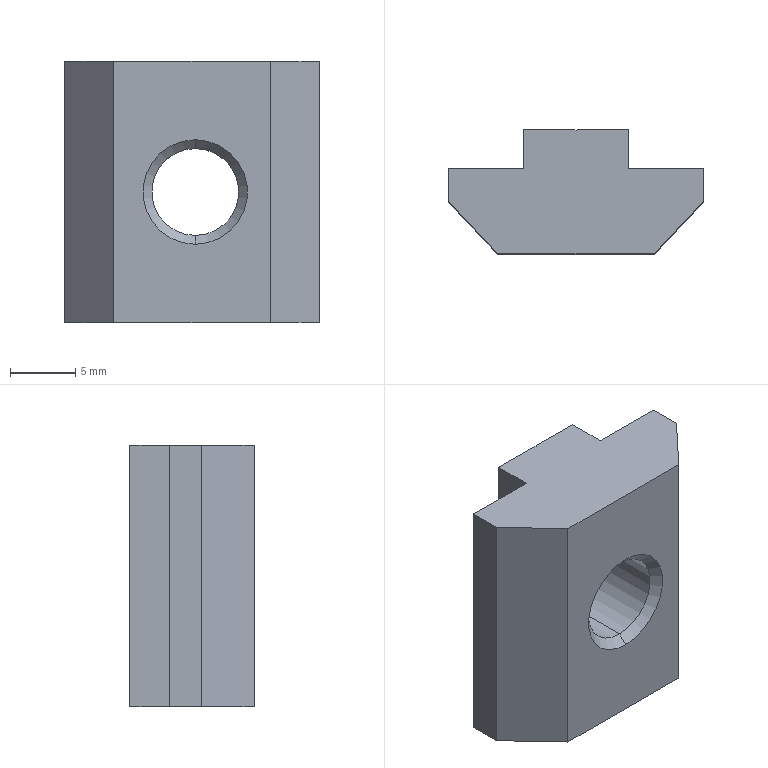Part | SolidWorks | features BaseBody 1 | 1 solid | 24 faces | box 19.5 x 9.5 x 20 mm | volume 2375 mm3 | plane 18 | cone 4 | cylinder 2 | commonest cylinder face diameters 6.647 x2
STEP:
#1=CARTESIAN_POINT('',(10.,0.6765,-6.676));
#2=VERTEX_POINT('',#1);
#3=CARTESIAN_POINT('',(10.,0.6765,-13.324));
#4=VERTEX_POINT('',#3);
#5=CARTESIAN_POINT('',(10.,0.6765,-10.));
#6=DIRECTION('',(0.,-1.,0.));
#7=DIRECTION('',(0.,0.,-1.));
#8=AXIS2_PLACEMENT_3D('',#5,#6,#7);
#9=CIRCLE('',#8,3.324);
#10=EDGE_CURVE('',#2,#4,#9,.T.);
#11=ORIENTED_EDGE('',*,*,#10,.F.);
#12=CARTESIAN_POINT('',(10.,0.,-6.));
#13=VERTEX_POINT('',#12);
#14=CARTESIAN_POINT('',(10.,0.,-6.));
#15=DIRECTION('',(0.,-0.7071,0.7071));
#16=VECTOR('',#15,1000.);
#17=LINE('',#14,#16);
#18=EDGE_CURVE('',#2,#13,#17,.T.);
#19=ORIENTED_EDGE('',*,*,#18,.T.);
#20=CARTESIAN_POINT('',(10.,0.,-14.));
#21=VERTEX_POINT('',#20);
#22=CARTESIAN_POINT('',(10.,0.,-10.));
#23=DIRECTION('',(0.,1.,0.));
#24=DIRECTION('',(0.,0.,-1.));
#25=AXIS2_PLACEMENT_3D('',#22,#23,#24);
#26=CIRCLE('',#25,4.);
#27=EDGE_CURVE('',#21,#13,#26,.T.);
#28=ORIENTED_EDGE('',*,*,#27,.F.);
#29=CARTESIAN_POINT('',(10.,0.,-14.));
#30=DIRECTION('',(0.,-0.7071,-0.7071));
#31=VECTOR('',#30,1000.);
#32=LINE('',#29,#31);
#33=EDGE_CURVE('',#4,#21,#32,.T.);
#34=ORIENTED_EDGE('',*,*,#33,.F.);
#35=EDGE_LOOP('',(#11,#19,#28,#34));
#36=FACE_OUTER_BOUND('',#35,.T.);
#37=CARTESIAN_POINT('',(10.,0.,-10.));
#38=DIRECTION('',(0.,-1.,0.));
#39=DIRECTION('',(0.,0.,-1.));
#40=AXIS2_PLACEMENT_3D('',#37,#38,#39);
#41=CONICAL_SURFACE('',#40,4.,0.7854);
#42=ADVANCED_FACE('',(#36),#41,.F.);
#43=ORIENTED_EDGE('',*,*,#10,.T.);
#44=CARTESIAN_POINT('',(10.,8.823,-13.324));
#45=VERTEX_POINT('',#44);
#46=CARTESIAN_POINT('',(10.,0.,-13.324));
#47=DIRECTION('',(0.,1.,0.));
#48=VECTOR('',#47,1000.);
#49=LINE('',#46,#48);
#50=EDGE_CURVE('',#4,#45,#49,.T.);
#51=ORIENTED_EDGE('',*,*,#50,.T.);
#52=CARTESIAN_POINT('',(10.,8.823,-6.676));
#53=VERTEX_POINT('',#52);
#54=CARTESIAN_POINT('',(10.,8.823,-10.));
#55=DIRECTION('',(0.,-1.,0.));
#56=DIRECTION('',(0.,0.,1.));
#57=AXIS2_PLACEMENT_3D('',#54,#55,#56);
#58=CIRCLE('',#57,3.324);
#59=EDGE_CURVE('',#53,#45,#58,.T.);
#60=ORIENTED_EDGE('',*,*,#59,.F.);
#61=CARTESIAN_POINT('',(10.,0.,-6.676));
#62=DIRECTION('',(0.,1.,0.));
#63=VECTOR('',#62,1000.);
#64=LINE('',#61,#63);
#65=EDGE_CURVE('',#2,#53,#64,.T.);
#66=ORIENTED_EDGE('',*,*,#65,.F.);
#67=EDGE_LOOP('',(#43,#51,#60,#66));
#68=FACE_OUTER_BOUND('',#67,.T.);
#69=CARTESIAN_POINT('',(10.,0.,-10.));
#70=DIRECTION('',(0.,1.,0.));
#71=DIRECTION('',(0.,0.,1.));
#72=AXIS2_PLACEMENT_3D('',#69,#70,#71);
#73=CYLINDRICAL_SURFACE('',#72,3.324);
#74=ADVANCED_FACE('',(#68),#73,.F.);
#75=ORIENTED_EDGE('',*,*,#59,.T.);
#76=CARTESIAN_POINT('',(10.,9.5,-14.));
#77=VERTEX_POINT('',#76);
#78=CARTESIAN_POINT('',(10.,9.5,-14.));
#79=DIRECTION('',(0.,0.7071,-0.7071));
#80=VECTOR('',#79,1000.);
#81=LINE('',#78,#80);
#82=EDGE_CURVE('',#45,#77,#81,.T.);
#83=ORIENTED_EDGE('',*,*,#82,.T.);
#84=CARTESIAN_POINT('',(9.85,9.5,-13.997));
#85=VERTEX_POINT('',#84);
#86=CARTESIAN_POINT('',(10.,9.5,-10.));
#87=DIRECTION('',(0.,-1.,0.));
#88=DIRECTION('',(0.,0.,1.));
#89=AXIS2_PLACEMENT_3D('',#86,#87,#88);
#90=CIRCLE('',#89,4.);
#91=EDGE_CURVE('',#85,#77,#90,.T.);
#92=ORIENTED_EDGE('',*,*,#91,.F.);
#93=CARTESIAN_POINT('',(9.75,9.42,-13.912));
#94=VERTEX_POINT('',#93);
#95=CARTESIAN_POINT('',(9.75,9.42,-13.912));
#96=CARTESIAN_POINT('',(9.783,9.446,-13.941));
#97=CARTESIAN_POINT('',(9.816,9.473,-13.969));
#98=CARTESIAN_POINT('',(9.85,9.5,-13.997));
#99=(BOUNDED_CURVE()B_SPLINE_CURVE(3,(#95,#96,#97,#98),.UNSPECIFIED.,.F.,.F.)B_SPLINE_CURVE_WITH_KNOTS((4,4),(3.748,3.763),.UNSPECIFIED.)CURVE()GEOMETRIC_REPRESENTATION_ITEM()RATIONAL_B_SPLINE_CURVE((1.,1.,1.,1.))REPRESENTATION_ITEM(''));
#100=EDGE_CURVE('',#94,#85,#99,.T.);
#101=ORIENTED_EDGE('',*,*,#100,.F.);
#102=CARTESIAN_POINT('',(9.65,9.5,-13.985));
#103=VERTEX_POINT('',#102);
#104=CARTESIAN_POINT('',(9.65,9.5,-13.985));
#105=CARTESIAN_POINT('',(9.684,9.473,-13.961));
#106=CARTESIAN_POINT('',(9.717,9.446,-13.936));
#107=CARTESIAN_POINT('',(9.75,9.42,-13.912));
#108=(BOUNDED_CURVE()B_SPLINE_CURVE(3,(#104,#105,#106,#107),.UNSPECIFIED.,.F.,.F.)B_SPLINE_CURVE_WITH_KNOTS((4,4),(2.444,2.459),.UNSPECIFIED.)CURVE()GEOMETRIC_REPRESENTATION_ITEM()RATIONAL_B_SPLINE_CURVE((1.,1.,1.,1.))REPRESENTATION_ITEM(''));
#109=EDGE_CURVE('',#103,#94,#108,.T.);
#110=ORIENTED_EDGE('',*,*,#109,.F.);
#111=CARTESIAN_POINT('',(9.65,9.5,-6.015));
#112=VERTEX_POINT('',#111);
#113=CARTESIAN_POINT('',(10.,9.5,-10.));
#114=DIRECTION('',(0.,-1.,0.));
#115=DIRECTION('',(0.,0.,1.));
#116=AXIS2_PLACEMENT_3D('',#113,#114,#115);
#117=CIRCLE('',#116,4.);
#118=EDGE_CURVE('',#112,#103,#117,.T.);
#119=ORIENTED_EDGE('',*,*,#118,.F.);
#120=CARTESIAN_POINT('',(9.75,9.42,-6.088));
#121=VERTEX_POINT('',#120);
#122=CARTESIAN_POINT('',(9.75,9.42,-6.088));
#123=CARTESIAN_POINT('',(9.717,9.446,-6.064));
#124=CARTESIAN_POINT('',(9.684,9.473,-6.039));
#125=CARTESIAN_POINT('',(9.65,9.5,-6.015));
#126=(BOUNDED_CURVE()B_SPLINE_CURVE(3,(#122,#123,#124,#125),.UNSPECIFIED.,.F.,.T.)B_SPLINE_CURVE_WITH_KNOTS((4,4),(3.824,3.84),.UNSPECIFIED.)CURVE()GEOMETRIC_REPRESENTATION_ITEM()RATIONAL_B_SPLINE_CURVE((1.,1.,1.,1.))REPRESENTATION_ITEM(''));
#127=EDGE_CURVE('',#121,#112,#126,.T.);
#128=ORIENTED_EDGE('',*,*,#127,.F.);
#129=CARTESIAN_POINT('',(9.85,9.5,-6.003));
#130=VERTEX_POINT('',#129);
#131=CARTESIAN_POINT('',(9.85,9.5,-6.003));
#132=CARTESIAN_POINT('',(9.816,9.473,-6.031));
#133=CARTESIAN_POINT('',(9.783,9.446,-6.059));
#134=CARTESIAN_POINT('',(9.75,9.42,-6.088));
#135=(BOUNDED_CURVE()B_SPLINE_CURVE(3,(#131,#132,#133,#134),.UNSPECIFIED.,.F.,.F.)B_SPLINE_CURVE_WITH_KNOTS((4,4),(2.52,2.535),.UNSPECIFIED.)CURVE()GEOMETRIC_REPRESENTATION_ITEM()RATIONAL_B_SPLINE_CURVE((1.,1.,1.,1.))REPRESENTATION_ITEM(''));
#136=EDGE_CURVE('',#130,#121,#135,.T.);
#137=ORIENTED_EDGE('',*,*,#136,.F.);
#138=CARTESIAN_POINT('',(10.,9.5,-6.));
#139=VERTEX_POINT('',#138);
#140=CARTESIAN_POINT('',(10.,9.5,-10.));
#141=DIRECTION('',(0.,-1.,0.));
#142=DIRECTION('',(0.,0.,1.));
#143=AXIS2_PLACEMENT_3D('',#140,#141,#142);
#144=CIRCLE('',#143,4.);
#145=EDGE_CURVE('',#139,#130,#144,.T.);
#146=ORIENTED_EDGE('',*,*,#145,.F.);
#147=CARTESIAN_POINT('',(10.,9.5,-6.));
#148=DIRECTION('',(0.,0.7071,0.7071));
#149=VECTOR('',#148,1000.);
#150=LINE('',#147,#149);
#151=EDGE_CURVE('',#53,#139,#150,.T.);
#152=ORIENTED_EDGE('',*,*,#151,.F.);
#153=EDGE_LOOP('',(#75,#83,#92,#101,#110,#119,#128,#137,#146,#152));
#154=FACE_OUTER_BOUND('',#153,.T.);
#155=CARTESIAN_POINT('',(10.,9.5,-10.));
#156=DIRECTION('',(0.,1.,0.));
#157=DIRECTION('',(0.,0.,1.));
#158=AXIS2_PLACEMENT_3D('',#155,#156,#157);
#159=CONICAL_SURFACE('',#158,4.,0.7854);
#160=ADVANCED_FACE('',(#154),#159,.F.);
#161=CARTESIAN_POINT('',(15.75,0.,0.));
#162=VERTEX_POINT('',#161);
#163=CARTESIAN_POINT('',(3.75,0.,0.));
#164=VERTEX_POINT('',#163);
#165=CARTESIAN_POINT('',(3.75,0.,0.));
#166=DIRECTION('',(-1.,0.,0.));
#167=VECTOR('',#166,1000.);
#168=LINE('',#165,#167);
#169=EDGE_CURVE('',#162,#164,#168,.T.);
#170=ORIENTED_EDGE('',*,*,#169,.T.);
#171=CARTESIAN_POINT('',(3.75,0.,-20.));
#172=VERTEX_POINT('',#171);
#173=CARTESIAN_POINT('',(3.75,0.,-20.));
#174=DIRECTION('',(0.,0.,-1.));
#175=VECTOR('',#174,1000.);
#176=LINE('',#173,#175);
#177=EDGE_CURVE('',#164,#172,#176,.T.);
#178=ORIENTED_EDGE('',*,*,#177,.T.);
#179=CARTESIAN_POINT('',(15.75,0.,-20.));
#180=VERTEX_POINT('',#179);
#181=CARTESIAN_POINT('',(3.75,0.,-20.));
#182=DIRECTION('',(1.,0.,0.));
#183=VECTOR('',#182,1000.);
#184=LINE('',#181,#183);
#185=EDGE_CURVE('',#172,#180,#184,.T.);
#186=ORIENTED_EDGE('',*,*,#185,.T.);
#187=CARTESIAN_POINT('',(15.75,0.,-20.));
#188=DIRECTION('',(0.,0.,1.));
#189=VECTOR('',#188,1000.);
#190=LINE('',#187,#189);
#191=EDGE_CURVE('',#180,#162,#190,.T.);
#192=ORIENTED_EDGE('',*,*,#191,.T.);
#193=EDGE_LOOP('',(#170,#178,#186,#192));
#194=FACE_OUTER_BOUND('',#193,.T.);
#195=ORIENTED_EDGE('',*,*,#27,.T.);
#196=CARTESIAN_POINT('',(10.,0.,-10.));
#197=DIRECTION('',(0.,1.,0.));
#198=DIRECTION('',(0.,0.,-1.));
#199=AXIS2_PLACEMENT_3D('',#196,#197,#198);
#200=CIRCLE('',#199,4.);
#201=EDGE_CURVE('',#13,#21,#200,.T.);
#202=ORIENTED_EDGE('',*,*,#201,.T.);
#203=EDGE_LOOP('',(#195,#202));
#204=FACE_BOUND('',#203,.T.);
#205=CARTESIAN_POINT('',(3.75,0.,-20.));
#206=DIRECTION('',(0.,-1.,0.));
#207=DIRECTION('',(0.,0.,-1.));
#208=AXIS2_PLACEMENT_3D('',#205,#206,#207);
#209=PLANE('',#208);
#210=ADVANCED_FACE('',(#194,#204),#209,.T.);
#211=CARTESIAN_POINT('',(0.,4.,0.));
#212=VERTEX_POINT('',#211);
#213=CARTESIAN_POINT('',(0.,4.,0.));
#214=DIRECTION('',(-0.6839,0.7295,0.));
#215=VECTOR('',#214,1000.);
#216=LINE('',#213,#215);
#217=EDGE_CURVE('',#164,#212,#216,.T.);
#218=ORIENTED_EDGE('',*,*,#217,.T.);
#219=CARTESIAN_POINT('',(0.,4.,-20.));
#220=VERTEX_POINT('',#219);
#221=CARTESIAN_POINT('',(0.,4.,-20.));
#222=DIRECTION('',(0.,0.,-1.));
#223=VECTOR('',#222,1000.);
#224=LINE('',#221,#223);
#225=EDGE_CURVE('',#212,#220,#224,.T.);
#226=ORIENTED_EDGE('',*,*,#225,.T.);
#227=CARTESIAN_POINT('',(0.,4.,-20.));
#228=DIRECTION('',(0.6839,-0.7295,0.));
#229=VECTOR('',#228,1000.);
#230=LINE('',#227,#229);
#231=EDGE_CURVE('',#220,#172,#230,.T.);
#232=ORIENTED_EDGE('',*,*,#231,.T.);
#233=ORIENTED_EDGE('',*,*,#177,.F.);
#234=EDGE_LOOP('',(#218,#226,#232,#233));
#235=FACE_OUTER_BOUND('',#234,.T.);
#236=CARTESIAN_POINT('',(0.,4.,-20.));
#237=DIRECTION('',(-0.7295,-0.6839,0.));
#238=DIRECTION('',(0.6839,-0.7295,0.));
#239=AXIS2_PLACEMENT_3D('',#236,#237,#238);
#240=PLANE('',#239);
#241=ADVANCED_FACE('',(#235),#240,.T.);
#242=CARTESIAN_POINT('',(9.75,9.42,0.));
#243=VERTEX_POINT('',#242);
#244=CARTESIAN_POINT('',(9.85,9.5,0.));
#245=VERTEX_POINT('',#244);
#246=CARTESIAN_POINT('',(9.85,9.5,0.));
#247=DIRECTION('',(0.7809,0.6247,0.));
#248=VECTOR('',#247,1000.);
#249=LINE('',#246,#248);
#250=EDGE_CURVE('',#243,#245,#249,.T.);
#251=ORIENTED_EDGE('',*,*,#250,.F.);
#252=CARTESIAN_POINT('',(9.65,9.5,0.));
#253=VERTEX_POINT('',#252);
#254=CARTESIAN_POINT('',(9.75,9.42,0.));
#255=DIRECTION('',(0.7809,-0.6247,0.));
#256=VECTOR('',#255,1000.);
#257=LINE('',#254,#256);
#258=EDGE_CURVE('',#253,#243,#257,.T.);
#259=ORIENTED_EDGE('',*,*,#258,.F.);
#260=CARTESIAN_POINT('',(5.75,9.5,0.));
#261=VERTEX_POINT('',#260);
#262=CARTESIAN_POINT('',(0.,9.5,0.));
#263=DIRECTION('',(-1.,0.,0.));
#264=VECTOR('',#263,1000.);
#265=LINE('',#262,#264);
#266=EDGE_CURVE('',#253,#261,#265,.T.);
#267=ORIENTED_EDGE('',*,*,#266,.T.);
#268=CARTESIAN_POINT('',(5.75,6.5,0.));
#269=VERTEX_POINT('',#268);
#270=CARTESIAN_POINT('',(5.75,0.,0.));
#271=DIRECTION('',(0.,-1.,0.));
#272=VECTOR('',#271,1000.);
#273=LINE('',#270,#272);
#274=EDGE_CURVE('',#261,#269,#273,.T.);
#275=ORIENTED_EDGE('',*,*,#274,.T.);
#276=CARTESIAN_POINT('',(0.,6.5,0.));
#277=VERTEX_POINT('',#276);
#278=CARTESIAN_POINT('',(0.,6.5,0.));
#279=DIRECTION('',(-1.,0.,0.));
#280=VECTOR('',#279,1000.);
#281=LINE('',#278,#280);
#282=EDGE_CURVE('',#269,#277,#281,.T.);
#283=ORIENTED_EDGE('',*,*,#282,.T.);
#284=CARTESIAN_POINT('',(0.,0.,0.));
#285=DIRECTION('',(0.,-1.,0.));
#286=VECTOR('',#285,1000.);
#287=LINE('',#284,#286);
#288=EDGE_CURVE('',#277,#212,#287,.T.);
#289=ORIENTED_EDGE('',*,*,#288,.T.);
#290=ORIENTED_EDGE('',*,*,#217,.F.);
#291=ORIENTED_EDGE('',*,*,#169,.F.);
#292=CARTESIAN_POINT('',(19.5,4.,0.));
#293=VERTEX_POINT('',#292);
#294=CARTESIAN_POINT('',(15.75,0.,0.));
#295=DIRECTION('',(0.6839,0.7295,0.));
#296=VECTOR('',#295,1000.);
#297=LINE('',#294,#296);
#298=EDGE_CURVE('',#162,#293,#297,.T.);
#299=ORIENTED_EDGE('',*,*,#298,.T.);
#300=CARTESIAN_POINT('',(19.5,6.5,0.));
#301=VERTEX_POINT('',#300);
#302=CARTESIAN_POINT('',(19.5,0.,0.));
#303=DIRECTION('',(0.,1.,0.));
#304=VECTOR('',#303,1000.);
#305=LINE('',#302,#304);
#306=EDGE_CURVE('',#293,#301,#305,.T.);
#307=ORIENTED_EDGE('',*,*,#306,.T.);
#308=CARTESIAN_POINT('',(13.75,6.5,0.));
#309=VERTEX_POINT('',#308);
#310=CARTESIAN_POINT('',(0.,6.5,0.));
#311=DIRECTION('',(-1.,0.,0.));
#312=VECTOR('',#311,1000.);
#313=LINE('',#310,#312);
#314=EDGE_CURVE('',#301,#309,#313,.T.);
#315=ORIENTED_EDGE('',*,*,#314,.T.);
#316=CARTESIAN_POINT('',(13.75,9.5,0.));
#317=VERTEX_POINT('',#316);
#318=CARTESIAN_POINT('',(13.75,0.,0.));
#319=DIRECTION('',(0.,1.,0.));
#320=VECTOR('',#319,1000.);
#321=LINE('',#318,#320);
#322=EDGE_CURVE('',#309,#317,#321,.T.);
#323=ORIENTED_EDGE('',*,*,#322,.T.);
#324=CARTESIAN_POINT('',(0.,9.5,0.));
#325=DIRECTION('',(-1.,0.,0.));
#326=VECTOR('',#325,1000.);
#327=LINE('',#324,#326);
#328=EDGE_CURVE('',#317,#245,#327,.T.);
#329=ORIENTED_EDGE('',*,*,#328,.T.);
#330=EDGE_LOOP('',(#251,#259,#267,#275,#283,#289,#290,#291,#299,#307,#315,#323,#329));
#331=FACE_OUTER_BOUND('',#330,.T.);
#332=CARTESIAN_POINT('',(0.,0.,0.));
#333=DIRECTION('',(0.,0.,1.));
#334=DIRECTION('',(1.,0.,0.));
#335=AXIS2_PLACEMENT_3D('',#332,#333,#334);
#336=PLANE('',#335);
#337=ADVANCED_FACE('',(#331),#336,.T.);
#338=ORIENTED_EDGE('',*,*,#298,.F.);
#339=ORIENTED_EDGE('',*,*,#191,.F.);
#340=CARTESIAN_POINT('',(19.5,4.,-20.));
#341=VERTEX_POINT('',#340);
#342=CARTESIAN_POINT('',(15.75,0.,-20.));
#343=DIRECTION('',(0.6839,0.7295,0.));
#344=VECTOR('',#343,1000.);
#345=LINE('',#342,#344);
#346=EDGE_CURVE('',#180,#341,#345,.T.);
#347=ORIENTED_EDGE('',*,*,#346,.T.);
#348=CARTESIAN_POINT('',(19.5,4.,-20.));
#349=DIRECTION('',(0.,0.,1.));
#350=VECTOR('',#349,1000.);
#351=LINE('',#348,#350);
#352=EDGE_CURVE('',#341,#293,#351,.T.);
#353=ORIENTED_EDGE('',*,*,#352,.T.);
#354=EDGE_LOOP('',(#338,#339,#347,#353));
#355=FACE_OUTER_BOUND('',#354,.T.);
#356=CARTESIAN_POINT('',(15.75,0.,-20.));
#357=DIRECTION('',(0.7295,-0.6839,0.));
#358=DIRECTION('',(0.6839,0.7295,0.));
#359=AXIS2_PLACEMENT_3D('',#356,#357,#358);
#360=PLANE('',#359);
#361=ADVANCED_FACE('',(#355),#360,.T.);
#362=CARTESIAN_POINT('',(9.65,9.5,-20.));
#363=VERTEX_POINT('',#362);
#364=CARTESIAN_POINT('',(5.75,9.5,-20.));
#365=VERTEX_POINT('',#364);
#366=CARTESIAN_POINT('',(0.,9.5,-20.));
#367=DIRECTION('',(-1.,0.,0.));
#368=VECTOR('',#367,1000.);
#369=LINE('',#366,#368);
#370=EDGE_CURVE('',#363,#365,#369,.T.);
#371=ORIENTED_EDGE('',*,*,#370,.F.);
#372=CARTESIAN_POINT('',(9.75,9.42,-20.));
#373=VERTEX_POINT('',#372);
#374=CARTESIAN_POINT('',(9.75,9.42,-20.));
#375=DIRECTION('',(-0.7809,0.6247,0.));
#376=VECTOR('',#375,1000.);
#377=LINE('',#374,#376);
#378=EDGE_CURVE('',#373,#363,#377,.T.);
#379=ORIENTED_EDGE('',*,*,#378,.F.);
#380=CARTESIAN_POINT('',(9.85,9.5,-20.));
#381=VERTEX_POINT('',#380);
#382=CARTESIAN_POINT('',(9.85,9.5,-20.));
#383=DIRECTION('',(-0.7809,-0.6247,0.));
#384=VECTOR('',#383,1000.);
#385=LINE('',#382,#384);
#386=EDGE_CURVE('',#381,#373,#385,.T.);
#387=ORIENTED_EDGE('',*,*,#386,.F.);
#388=CARTESIAN_POINT('',(13.75,9.5,-20.));
#389=VERTEX_POINT('',#388);
#390=CARTESIAN_POINT('',(0.,9.5,-20.));
#391=DIRECTION('',(-1.,0.,0.));
#392=VECTOR('',#391,1000.);
#393=LINE('',#390,#392);
#394=EDGE_CURVE('',#389,#381,#393,.T.);
#395=ORIENTED_EDGE('',*,*,#394,.F.);
#396=CARTESIAN_POINT('',(13.75,6.5,-20.));
#397=VERTEX_POINT('',#396);
#398=CARTESIAN_POINT('',(13.75,0.,-20.));
#399=DIRECTION('',(0.,1.,0.));
#400=VECTOR('',#399,1000.);
#401=LINE('',#398,#400);
#402=EDGE_CURVE('',#397,#389,#401,.T.);
#403=ORIENTED_EDGE('',*,*,#402,.F.);
#404=CARTESIAN_POINT('',(19.5,6.5,-20.));
#405=VERTEX_POINT('',#404);
#406=CARTESIAN_POINT('',(0.,6.5,-20.));
#407=DIRECTION('',(-1.,0.,0.));
#408=VECTOR('',#407,1000.);
#409=LINE('',#406,#408);
#410=EDGE_CURVE('',#405,#397,#409,.T.);
#411=ORIENTED_EDGE('',*,*,#410,.F.);
#412=CARTESIAN_POINT('',(19.5,0.,-20.));
#413=DIRECTION('',(0.,1.,0.));
#414=VECTOR('',#413,1000.);
#415=LINE('',#412,#414);
#416=EDGE_CURVE('',#341,#405,#415,.T.);
#417=ORIENTED_EDGE('',*,*,#416,.F.);
#418=ORIENTED_EDGE('',*,*,#346,.F.);
#419=ORIENTED_EDGE('',*,*,#185,.F.);
#420=ORIENTED_EDGE('',*,*,#231,.F.);
#421=CARTESIAN_POINT('',(0.,6.5,-20.));
#422=VERTEX_POINT('',#421);
#423=CARTESIAN_POINT('',(0.,0.,-20.));
#424=DIRECTION('',(0.,-1.,0.));
#425=VECTOR('',#424,1000.);
#426=LINE('',#423,#425);
#427=EDGE_CURVE('',#422,#220,#426,.T.);
#428=ORIENTED_EDGE('',*,*,#427,.F.);
#429=CARTESIAN_POINT('',(5.75,6.5,-20.));
#430=VERTEX_POINT('',#429);
#431=CARTESIAN_POINT('',(0.,6.5,-20.));
#432=DIRECTION('',(-1.,0.,0.));
#433=VECTOR('',#432,1000.);
#434=LINE('',#431,#433);
#435=EDGE_CURVE('',#430,#422,#434,.T.);
#436=ORIENTED_EDGE('',*,*,#435,.F.);
#437=CARTESIAN_POINT('',(5.75,0.,-20.));
#438=DIRECTION('',(0.,-1.,0.));
#439=VECTOR('',#438,1000.);
#440=LINE('',#437,#439);
#441=EDGE_CURVE('',#365,#430,#440,.T.);
#442=ORIENTED_EDGE('',*,*,#441,.F.);
#443=EDGE_LOOP('',(#371,#379,#387,#395,#403,#411,#417,#418,#419,#420,#428,#436,#442));
#444=FACE_OUTER_BOUND('',#443,.T.);
#445=CARTESIAN_POINT('',(0.,0.,-20.));
#446=DIRECTION('',(0.,0.,1.));
#447=DIRECTION('',(1.,0.,0.));
#448=AXIS2_PLACEMENT_3D('',#445,#446,#447);
#449=PLANE('',#448);
#450=ADVANCED_FACE('',(#444),#449,.F.);
#451=ORIENTED_EDGE('',*,*,#18,.F.);
#452=CARTESIAN_POINT('',(10.,0.6765,-10.));
#453=DIRECTION('',(0.,-1.,0.));
#454=DIRECTION('',(0.,0.,-1.));
#455=AXIS2_PLACEMENT_3D('',#452,#453,#454);
#456=CIRCLE('',#455,3.324);
#457=EDGE_CURVE('',#4,#2,#456,.T.);
#458=ORIENTED_EDGE('',*,*,#457,.F.);
#459=ORIENTED_EDGE('',*,*,#33,.T.);
#460=ORIENTED_EDGE('',*,*,#201,.F.);
#461=EDGE_LOOP('',(#451,#458,#459,#460));
#462=FACE_OUTER_BOUND('',#461,.T.);
#463=CARTESIAN_POINT('',(10.,0.,-10.));
#464=DIRECTION('',(0.,-1.,0.));
#465=DIRECTION('',(0.,0.,-1.));
#466=AXIS2_PLACEMENT_3D('',#463,#464,#465);
#467=CONICAL_SURFACE('',#466,4.,0.7854);
#468=ADVANCED_FACE('',(#462),#467,.F.);
#469=ORIENTED_EDGE('',*,*,#288,.F.);
#470=CARTESIAN_POINT('',(0.,6.5,-20.));
#471=DIRECTION('',(0.,0.,-1.));
#472=VECTOR('',#471,1000.);
#473=LINE('',#470,#472);
#474=EDGE_CURVE('',#277,#422,#473,.T.);
#475=ORIENTED_EDGE('',*,*,#474,.T.);
#476=ORIENTED_EDGE('',*,*,#427,.T.);
#477=ORIENTED_EDGE('',*,*,#225,.F.);
#478=EDGE_LOOP('',(#469,#475,#476,#477));
#479=FACE_OUTER_BOUND('',#478,.T.);
#480=CARTESIAN_POINT('',(0.,6.5,-20.));
#481=DIRECTION('',(-1.,0.,0.));
#482=DIRECTION('',(0.,0.,1.));
#483=AXIS2_PLACEMENT_3D('',#480,#481,#482);
#484=PLANE('',#483);
#485=ADVANCED_FACE('',(#479),#484,.T.);
#486=CARTESIAN_POINT('',(13.75,9.5,-8.608));
#487=VERTEX_POINT('',#486);
#488=CARTESIAN_POINT('',(10.,9.5,-10.));
#489=DIRECTION('',(0.,-1.,0.));
#490=DIRECTION('',(0.,0.,1.));
#491=AXIS2_PLACEMENT_3D('',#488,#489,#490);
#492=CIRCLE('',#491,4.);
#493=EDGE_CURVE('',#487,#139,#492,.T.);
#494=ORIENTED_EDGE('',*,*,#493,.T.);
#495=ORIENTED_EDGE('',*,*,#145,.T.);
#496=CARTESIAN_POINT('',(9.85,9.5,-20.));
#497=DIRECTION('',(0.,0.,1.));
#498=VECTOR('',#497,1000.);
#499=LINE('',#496,#498);
#500=EDGE_CURVE('',#130,#245,#499,.T.);
#501=ORIENTED_EDGE('',*,*,#500,.T.);
#502=ORIENTED_EDGE('',*,*,#328,.F.);
#503=CARTESIAN_POINT('',(13.75,9.5,-20.));
#504=DIRECTION('',(0.,0.,-1.));
#505=VECTOR('',#504,1000.);
#506=LINE('',#503,#505);
#507=EDGE_CURVE('',#317,#487,#506,.T.);
#508=ORIENTED_EDGE('',*,*,#507,.T.);
#509=EDGE_LOOP('',(#494,#495,#501,#502,#508));
#510=FACE_OUTER_BOUND('',#509,.T.);
#511=CARTESIAN_POINT('',(13.75,9.5,-20.));
#512=DIRECTION('',(0.,1.,0.));
#513=DIRECTION('',(0.,0.,1.));
#514=AXIS2_PLACEMENT_3D('',#511,#512,#513);
#515=PLANE('',#514);
#516=ADVANCED_FACE('',(#510),#515,.T.);
#517=ORIENTED_EDGE('',*,*,#507,.F.);
#518=ORIENTED_EDGE('',*,*,#322,.F.);
#519=CARTESIAN_POINT('',(13.75,6.5,-20.));
#520=DIRECTION('',(0.,0.,-1.));
#521=VECTOR('',#520,1000.);
#522=LINE('',#519,#521);
#523=EDGE_CURVE('',#309,#397,#522,.T.);
#524=ORIENTED_EDGE('',*,*,#523,.T.);
#525=ORIENTED_EDGE('',*,*,#402,.T.);
#526=CARTESIAN_POINT('',(13.75,9.5,-11.392));
#527=VERTEX_POINT('',#526);
#528=CARTESIAN_POINT('',(13.75,9.5,-20.));
#529=DIRECTION('',(0.,0.,1.));
#530=VECTOR('',#529,1000.);
#531=LINE('',#528,#530);
#532=EDGE_CURVE('',#389,#527,#531,.T.);
#533=ORIENTED_EDGE('',*,*,#532,.T.);
#534=CARTESIAN_POINT('',(13.75,9.5,-11.392));
#535=CARTESIAN_POINT('',(13.75,9.343,-10.941));
#536=CARTESIAN_POINT('',(13.75,9.25,-10.48));
#537=CARTESIAN_POINT('',(13.75,9.25,-9.524));
#538=CARTESIAN_POINT('',(13.75,9.343,-9.059));
#539=CARTESIAN_POINT('',(13.75,9.5,-8.608));
#540=B_SPLINE_CURVE_WITH_KNOTS('',3,(#534,#535,#536,#537,#538,#539),.UNSPECIFIED.,.F.,.F.,(4,2,4),(0.,0.001412,0.002825),.UNSPECIFIED.);
#541=EDGE_CURVE('',#527,#487,#540,.T.);
#542=ORIENTED_EDGE('',*,*,#541,.T.);
#543=EDGE_LOOP('',(#517,#518,#524,#525,#533,#542));
#544=FACE_OUTER_BOUND('',#543,.T.);
#545=CARTESIAN_POINT('',(13.75,6.5,-20.));
#546=DIRECTION('',(1.,0.,0.));
#547=DIRECTION('',(0.,0.,-1.));
#548=AXIS2_PLACEMENT_3D('',#545,#546,#547);
#549=PLANE('',#548);
#550=ADVANCED_FACE('',(#544),#549,.T.);
#551=ORIENTED_EDGE('',*,*,#314,.F.);
#552=CARTESIAN_POINT('',(19.5,6.5,-20.));
#553=DIRECTION('',(0.,0.,-1.));
#554=VECTOR('',#553,1000.);
#555=LINE('',#552,#554);
#556=EDGE_CURVE('',#301,#405,#555,.T.);
#557=ORIENTED_EDGE('',*,*,#556,.T.);
#558=ORIENTED_EDGE('',*,*,#410,.T.);
#559=ORIENTED_EDGE('',*,*,#523,.F.);
#560=EDGE_LOOP('',(#551,#557,#558,#559));
#561=FACE_OUTER_BOUND('',#560,.T.);
#562=CARTESIAN_POINT('',(19.5,6.5,-20.));
#563=DIRECTION('',(0.,1.,0.));
#564=DIRECTION('',(0.,0.,1.));
#565=AXIS2_PLACEMENT_3D('',#562,#563,#564);
#566=PLANE('',#565);
#567=ADVANCED_FACE('',(#561),#566,.T.);
#568=ORIENTED_EDGE('',*,*,#306,.F.);
#569=ORIENTED_EDGE('',*,*,#352,.F.);
#570=ORIENTED_EDGE('',*,*,#416,.T.);
#571=ORIENTED_EDGE('',*,*,#556,.F.);
#572=EDGE_LOOP('',(#568,#569,#570,#571));
#573=FACE_OUTER_BOUND('',#572,.T.);
#574=CARTESIAN_POINT('',(19.5,4.,-20.));
#575=DIRECTION('',(1.,0.,0.));
#576=DIRECTION('',(0.,0.,-1.));
#577=AXIS2_PLACEMENT_3D('',#574,#575,#576);
#578=PLANE('',#577);
#579=ADVANCED_FACE('',(#573),#578,.T.);
#580=ORIENTED_EDGE('',*,*,#282,.F.);
#581=CARTESIAN_POINT('',(5.75,6.5,-20.));
#582=DIRECTION('',(0.,0.,-1.));
#583=VECTOR('',#582,1000.);
#584=LINE('',#581,#583);
#585=EDGE_CURVE('',#269,#430,#584,.T.);
#586=ORIENTED_EDGE('',*,*,#585,.T.);
#587=ORIENTED_EDGE('',*,*,#435,.T.);
#588=ORIENTED_EDGE('',*,*,#474,.F.);
#589=EDGE_LOOP('',(#580,#586,#587,#588));
#590=FACE_OUTER_BOUND('',#589,.T.);
#591=CARTESIAN_POINT('',(5.75,6.5,-20.));
#592=DIRECTION('',(0.,1.,0.));
#593=DIRECTION('',(0.,0.,1.));
#594=AXIS2_PLACEMENT_3D('',#591,#592,#593);
#595=PLANE('',#594);
#596=ADVANCED_FACE('',(#590),#595,.T.);
#597=ORIENTED_EDGE('',*,*,#274,.F.);
#598=CARTESIAN_POINT('',(5.75,9.5,-20.));
#599=DIRECTION('',(0.,0.,-1.));
#600=VECTOR('',#599,1000.);
#601=LINE('',#598,#600);
#602=EDGE_CURVE('',#261,#365,#601,.T.);
#603=ORIENTED_EDGE('',*,*,#602,.T.);
#604=ORIENTED_EDGE('',*,*,#441,.T.);
#605=ORIENTED_EDGE('',*,*,#585,.F.);
#606=EDGE_LOOP('',(#597,#603,#604,#605));
#607=FACE_OUTER_BOUND('',#606,.T.);
#608=CARTESIAN_POINT('',(5.75,9.5,-20.));
#609=DIRECTION('',(-1.,0.,0.));
#610=DIRECTION('',(0.,0.,1.));
#611=AXIS2_PLACEMENT_3D('',#608,#609,#610);
#612=PLANE('',#611);
#613=ADVANCED_FACE('',(#607),#612,.T.);
#614=CARTESIAN_POINT('',(9.65,9.5,-20.));
#615=DIRECTION('',(0.,0.,-1.));
#616=VECTOR('',#615,1000.);
#617=LINE('',#614,#616);
#618=EDGE_CURVE('',#103,#363,#617,.T.);
#619=ORIENTED_EDGE('',*,*,#618,.T.);
#620=ORIENTED_EDGE('',*,*,#370,.T.);
#621=ORIENTED_EDGE('',*,*,#602,.F.);
#622=ORIENTED_EDGE('',*,*,#266,.F.);
#623=CARTESIAN_POINT('',(9.65,9.5,-20.));
#624=DIRECTION('',(0.,0.,-1.));
#625=VECTOR('',#624,1000.);
#626=LINE('',#623,#625);
#627=EDGE_CURVE('',#253,#112,#626,.T.);
#628=ORIENTED_EDGE('',*,*,#627,.T.);
#629=ORIENTED_EDGE('',*,*,#118,.T.);
#630=EDGE_LOOP('',(#619,#620,#621,#622,#628,#629));
#631=FACE_OUTER_BOUND('',#630,.T.);
#632=CARTESIAN_POINT('',(9.65,9.5,-20.));
#633=DIRECTION('',(0.,1.,0.));
#634=DIRECTION('',(0.,0.,1.));
#635=AXIS2_PLACEMENT_3D('',#632,#633,#634);
#636=PLANE('',#635);
#637=ADVANCED_FACE('',(#631),#636,.T.);
#638=CARTESIAN_POINT('',(9.85,9.5,-20.));
#639=DIRECTION('',(0.,0.,1.));
#640=VECTOR('',#639,1000.);
#641=LINE('',#638,#640);
#642=EDGE_CURVE('',#381,#85,#641,.T.);
#643=ORIENTED_EDGE('',*,*,#642,.T.);
#644=ORIENTED_EDGE('',*,*,#91,.T.);
#645=CARTESIAN_POINT('',(10.,9.5,-10.));
#646=DIRECTION('',(0.,-1.,0.));
#647=DIRECTION('',(0.,0.,1.));
#648=AXIS2_PLACEMENT_3D('',#645,#646,#647);
#649=CIRCLE('',#648,4.);
#650=EDGE_CURVE('',#77,#527,#649,.T.);
#651=ORIENTED_EDGE('',*,*,#650,.T.);
#652=ORIENTED_EDGE('',*,*,#532,.F.);
#653=ORIENTED_EDGE('',*,*,#394,.T.);
#654=EDGE_LOOP('',(#643,#644,#651,#652,#653));
#655=FACE_OUTER_BOUND('',#654,.T.);
#656=CARTESIAN_POINT('',(13.75,9.5,-20.));
#657=DIRECTION('',(0.,1.,0.));
#658=DIRECTION('',(0.,0.,1.));
#659=AXIS2_PLACEMENT_3D('',#656,#657,#658);
#660=PLANE('',#659);
#661=ADVANCED_FACE('',(#655),#660,.T.);
#662=ORIENTED_EDGE('',*,*,#50,.F.);
#663=ORIENTED_EDGE('',*,*,#457,.T.);
#664=ORIENTED_EDGE('',*,*,#65,.T.);
#665=CARTESIAN_POINT('',(10.,8.823,-10.));
#666=DIRECTION('',(0.,-1.,0.));
#667=DIRECTION('',(0.,0.,1.));
#668=AXIS2_PLACEMENT_3D('',#665,#666,#667);
#669=CIRCLE('',#668,3.324);
#670=EDGE_CURVE('',#45,#53,#669,.T.);
#671=ORIENTED_EDGE('',*,*,#670,.F.);
#672=EDGE_LOOP('',(#662,#663,#664,#671));
#673=FACE_OUTER_BOUND('',#672,.T.);
#674=CARTESIAN_POINT('',(10.,0.,-10.));
#675=DIRECTION('',(0.,1.,0.));
#676=DIRECTION('',(0.,0.,1.));
#677=AXIS2_PLACEMENT_3D('',#674,#675,#676);
#678=CYLINDRICAL_SURFACE('',#677,3.324);
#679=ADVANCED_FACE('',(#673),#678,.F.);
#680=ORIENTED_EDGE('',*,*,#82,.F.);
#681=ORIENTED_EDGE('',*,*,#670,.T.);
#682=ORIENTED_EDGE('',*,*,#151,.T.);
#683=ORIENTED_EDGE('',*,*,#493,.F.);
#684=ORIENTED_EDGE('',*,*,#541,.F.);
#685=ORIENTED_EDGE('',*,*,#650,.F.);
#686=EDGE_LOOP('',(#680,#681,#682,#683,#684,#685));
#687=FACE_OUTER_BOUND('',#686,.T.);
#688=CARTESIAN_POINT('',(10.,9.5,-10.));
#689=DIRECTION('',(0.,1.,0.));
#690=DIRECTION('',(0.,0.,1.));
#691=AXIS2_PLACEMENT_3D('',#688,#689,#690);
#692=CONICAL_SURFACE('',#691,4.,0.7854);
#693=ADVANCED_FACE('',(#687),#692,.F.);
#694=ORIENTED_EDGE('',*,*,#500,.F.);
#695=ORIENTED_EDGE('',*,*,#136,.T.);
#696=CARTESIAN_POINT('',(9.75,9.42,-20.));
#697=DIRECTION('',(0.,0.,1.));
#698=VECTOR('',#697,1000.);
#699=LINE('',#696,#698);
#700=EDGE_CURVE('',#121,#243,#699,.T.);
#701=ORIENTED_EDGE('',*,*,#700,.T.);
#702=ORIENTED_EDGE('',*,*,#250,.T.);
#703=EDGE_LOOP('',(#694,#695,#701,#702));
#704=FACE_OUTER_BOUND('',#703,.T.);
#705=CARTESIAN_POINT('',(9.85,9.5,-20.));
#706=DIRECTION('',(-0.6247,0.7809,0.));
#707=DIRECTION('',(-0.7809,-0.6247,0.));
#708=AXIS2_PLACEMENT_3D('',#705,#706,#707);
#709=PLANE('',#708);
#710=ADVANCED_FACE('',(#704),#709,.T.);
#711=ORIENTED_EDGE('',*,*,#618,.F.);
#712=ORIENTED_EDGE('',*,*,#109,.T.);
#713=CARTESIAN_POINT('',(9.75,9.42,-20.));
#714=DIRECTION('',(0.,0.,-1.));
#715=VECTOR('',#714,1000.);
#716=LINE('',#713,#715);
#717=EDGE_CURVE('',#94,#373,#716,.T.);
#718=ORIENTED_EDGE('',*,*,#717,.T.);
#719=ORIENTED_EDGE('',*,*,#378,.T.);
#720=EDGE_LOOP('',(#711,#712,#718,#719));
#721=FACE_OUTER_BOUND('',#720,.T.);
#722=CARTESIAN_POINT('',(9.75,9.42,-20.));
#723=DIRECTION('',(0.6247,0.7809,0.));
#724=DIRECTION('',(-0.7809,0.6247,0.));
#725=AXIS2_PLACEMENT_3D('',#722,#723,#724);
#726=PLANE('',#725);
#727=ADVANCED_FACE('',(#721),#726,.T.);
#728=ORIENTED_EDGE('',*,*,#700,.F.);
#729=ORIENTED_EDGE('',*,*,#127,.T.);
#730=ORIENTED_EDGE('',*,*,#627,.F.);
#731=ORIENTED_EDGE('',*,*,#258,.T.);
#732=EDGE_LOOP('',(#728,#729,#730,#731));
#733=FACE_OUTER_BOUND('',#732,.T.);
#734=CARTESIAN_POINT('',(9.75,9.42,-20.));
#735=DIRECTION('',(0.6247,0.7809,0.));
#736=DIRECTION('',(-0.7809,0.6247,0.));
#737=AXIS2_PLACEMENT_3D('',#734,#735,#736);
#738=PLANE('',#737);
#739=ADVANCED_FACE('',(#733),#738,.T.);
#740=ORIENTED_EDGE('',*,*,#717,.F.);
#741=ORIENTED_EDGE('',*,*,#100,.T.);
#742=ORIENTED_EDGE('',*,*,#642,.F.);
#743=ORIENTED_EDGE('',*,*,#386,.T.);
#744=EDGE_LOOP('',(#740,#741,#742,#743));
#745=FACE_OUTER_BOUND('',#744,.T.);
#746=CARTESIAN_POINT('',(9.85,9.5,-20.));
#747=DIRECTION('',(-0.6247,0.7809,0.));
#748=DIRECTION('',(-0.7809,-0.6247,0.));
#749=AXIS2_PLACEMENT_3D('',#746,#747,#748);
#750=PLANE('',#749);
#751=ADVANCED_FACE('',(#745),#750,.T.);
#752=CLOSED_SHELL('',(#42,#74,#160,#210,#241,#337,#361,#450,#468,#485,#516,#550,#567,#579,#596,#613,#637,#661,#679,#693,#710,#727,#739,#751));
#753=MANIFOLD_SOLID_BREP('',#752);
#754=CARTESIAN_POINT('',(0.,0.,0.));
#755=DIRECTION('',(0.,0.,1.));
#756=DIRECTION('',(1.,0.,0.));
#757=AXIS2_PLACEMENT_3D('',#754,#755,#756);
#758=(LENGTH_UNIT()NAMED_UNIT(*)SI_UNIT(.MILLI.,.METRE.));
#759=UNCERTAINTY_MEASURE_WITH_UNIT(LENGTH_MEASURE(0.00001),#758,'','');
#760=(NAMED_UNIT(*)PLANE_ANGLE_UNIT()SI_UNIT($,.RADIAN.));
#761=(NAMED_UNIT(*)SI_UNIT($,.STERADIAN.)SOLID_ANGLE_UNIT());
#762=(GEOMETRIC_REPRESENTATION_CONTEXT(3)GLOBAL_UNCERTAINTY_ASSIGNED_CONTEXT((#759))GLOBAL_UNIT_ASSIGNED_CONTEXT((#758,#760,#761))REPRESENTATION_CONTEXT('',''));
#763=ADVANCED_BREP_SHAPE_REPRESENTATION('',(#753,#757),#762);